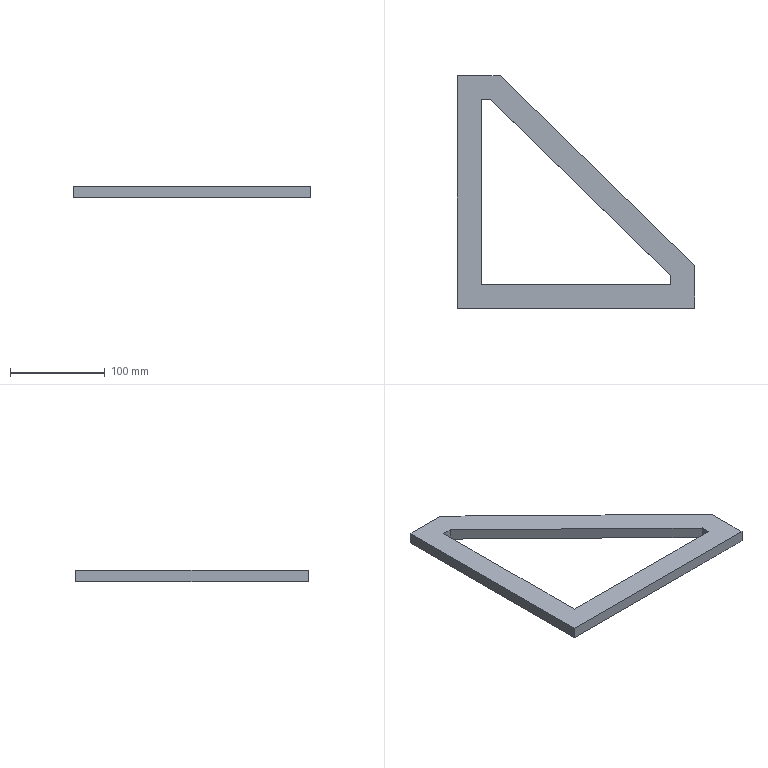Part | SolidWorks | features Extrusion 1 | 1 solid | 12 faces | box 250 x 245 x 12 mm | volume 232707 mm3 | plane 12
STEP:
#1=CARTESIAN_POINT('',(0.,0.,6.));
#2=VERTEX_POINT('',#1);
#3=CARTESIAN_POINT('',(0.,45.,6.));
#4=VERTEX_POINT('',#3);
#5=CARTESIAN_POINT('',(0.,45.,6.));
#6=DIRECTION('',(0.,1.,0.));
#7=VECTOR('',#6,1000.);
#8=LINE('',#5,#7);
#9=EDGE_CURVE('',#2,#4,#8,.T.);
#10=ORIENTED_EDGE('',*,*,#9,.T.);
#11=CARTESIAN_POINT('',(-205.,245.,6.));
#12=VERTEX_POINT('',#11);
#13=CARTESIAN_POINT('',(-205.,245.,6.));
#14=DIRECTION('',(-0.7158,0.6983,0.));
#15=VECTOR('',#14,1000.);
#16=LINE('',#13,#15);
#17=EDGE_CURVE('',#4,#12,#16,.T.);
#18=ORIENTED_EDGE('',*,*,#17,.T.);
#19=CARTESIAN_POINT('',(-250.,245.,6.));
#20=VERTEX_POINT('',#19);
#21=CARTESIAN_POINT('',(-250.,245.,6.));
#22=DIRECTION('',(-1.,0.,0.));
#23=VECTOR('',#22,1000.);
#24=LINE('',#21,#23);
#25=EDGE_CURVE('',#12,#20,#24,.T.);
#26=ORIENTED_EDGE('',*,*,#25,.T.);
#27=CARTESIAN_POINT('',(-250.,0.,6.));
#28=VERTEX_POINT('',#27);
#29=CARTESIAN_POINT('',(-250.,0.,6.));
#30=DIRECTION('',(0.,-1.,0.));
#31=VECTOR('',#30,1000.);
#32=LINE('',#29,#31);
#33=EDGE_CURVE('',#20,#28,#32,.T.);
#34=ORIENTED_EDGE('',*,*,#33,.T.);
#35=CARTESIAN_POINT('',(0.,0.,6.));
#36=DIRECTION('',(1.,0.,0.));
#37=VECTOR('',#36,1000.);
#38=LINE('',#35,#37);
#39=EDGE_CURVE('',#28,#2,#38,.T.);
#40=ORIENTED_EDGE('',*,*,#39,.T.);
#41=EDGE_LOOP('',(#10,#18,#26,#34,#40));
#42=FACE_OUTER_BOUND('',#41,.T.);
#43=CARTESIAN_POINT('',(-225.,220.,6.));
#44=VERTEX_POINT('',#43);
#45=CARTESIAN_POINT('',(-225.,25.,6.));
#46=VERTEX_POINT('',#45);
#47=CARTESIAN_POINT('',(-225.,25.,6.));
#48=DIRECTION('',(0.,-1.,0.));
#49=VECTOR('',#48,1000.);
#50=LINE('',#47,#49);
#51=EDGE_CURVE('',#44,#46,#50,.T.);
#52=ORIENTED_EDGE('',*,*,#51,.F.);
#53=CARTESIAN_POINT('',(-215.175,220.,6.));
#54=VERTEX_POINT('',#53);
#55=CARTESIAN_POINT('',(-225.,220.,6.));
#56=DIRECTION('',(-1.,0.,0.));
#57=VECTOR('',#56,1000.);
#58=LINE('',#55,#57);
#59=EDGE_CURVE('',#54,#44,#58,.T.);
#60=ORIENTED_EDGE('',*,*,#59,.F.);
#61=CARTESIAN_POINT('',(-25.,34.463,6.));
#62=VERTEX_POINT('',#61);
#63=CARTESIAN_POINT('',(-215.175,220.,6.));
#64=DIRECTION('',(-0.7158,0.6983,0.));
#65=VECTOR('',#64,1000.);
#66=LINE('',#63,#65);
#67=EDGE_CURVE('',#62,#54,#66,.T.);
#68=ORIENTED_EDGE('',*,*,#67,.F.);
#69=CARTESIAN_POINT('',(-25.,25.,6.));
#70=VERTEX_POINT('',#69);
#71=CARTESIAN_POINT('',(-25.,34.463,6.));
#72=DIRECTION('',(0.,1.,0.));
#73=VECTOR('',#72,1000.);
#74=LINE('',#71,#73);
#75=EDGE_CURVE('',#70,#62,#74,.T.);
#76=ORIENTED_EDGE('',*,*,#75,.F.);
#77=CARTESIAN_POINT('',(-25.,25.,6.));
#78=DIRECTION('',(1.,0.,0.));
#79=VECTOR('',#78,1000.);
#80=LINE('',#77,#79);
#81=EDGE_CURVE('',#46,#70,#80,.T.);
#82=ORIENTED_EDGE('',*,*,#81,.F.);
#83=EDGE_LOOP('',(#52,#60,#68,#76,#82));
#84=FACE_BOUND('',#83,.T.);
#85=CARTESIAN_POINT('',(0.,0.,6.));
#86=DIRECTION('',(0.,0.,-1.));
#87=DIRECTION('',(-1.,0.,0.));
#88=AXIS2_PLACEMENT_3D('',#85,#86,#87);
#89=PLANE('',#88);
#90=ADVANCED_FACE('',(#42,#84),#89,.F.);
#91=CARTESIAN_POINT('',(0.,0.,-6.));
#92=VERTEX_POINT('',#91);
#93=CARTESIAN_POINT('',(0.,45.,-6.));
#94=VERTEX_POINT('',#93);
#95=CARTESIAN_POINT('',(0.,45.,-6.));
#96=DIRECTION('',(0.,1.,0.));
#97=VECTOR('',#96,1000.);
#98=LINE('',#95,#97);
#99=EDGE_CURVE('',#92,#94,#98,.T.);
#100=ORIENTED_EDGE('',*,*,#99,.F.);
#101=CARTESIAN_POINT('',(-250.,0.,-6.));
#102=VERTEX_POINT('',#101);
#103=CARTESIAN_POINT('',(0.,0.,-6.));
#104=DIRECTION('',(1.,0.,0.));
#105=VECTOR('',#104,1000.);
#106=LINE('',#103,#105);
#107=EDGE_CURVE('',#102,#92,#106,.T.);
#108=ORIENTED_EDGE('',*,*,#107,.F.);
#109=CARTESIAN_POINT('',(-250.,245.,-6.));
#110=VERTEX_POINT('',#109);
#111=CARTESIAN_POINT('',(-250.,0.,-6.));
#112=DIRECTION('',(0.,-1.,0.));
#113=VECTOR('',#112,1000.);
#114=LINE('',#111,#113);
#115=EDGE_CURVE('',#110,#102,#114,.T.);
#116=ORIENTED_EDGE('',*,*,#115,.F.);
#117=CARTESIAN_POINT('',(-205.,245.,-6.));
#118=VERTEX_POINT('',#117);
#119=CARTESIAN_POINT('',(-250.,245.,-6.));
#120=DIRECTION('',(-1.,0.,0.));
#121=VECTOR('',#120,1000.);
#122=LINE('',#119,#121);
#123=EDGE_CURVE('',#118,#110,#122,.T.);
#124=ORIENTED_EDGE('',*,*,#123,.F.);
#125=CARTESIAN_POINT('',(-205.,245.,-6.));
#126=DIRECTION('',(-0.7158,0.6983,0.));
#127=VECTOR('',#126,1000.);
#128=LINE('',#125,#127);
#129=EDGE_CURVE('',#94,#118,#128,.T.);
#130=ORIENTED_EDGE('',*,*,#129,.F.);
#131=EDGE_LOOP('',(#100,#108,#116,#124,#130));
#132=FACE_OUTER_BOUND('',#131,.T.);
#133=CARTESIAN_POINT('',(-215.175,220.,-6.));
#134=VERTEX_POINT('',#133);
#135=CARTESIAN_POINT('',(-225.,220.,-6.));
#136=VERTEX_POINT('',#135);
#137=CARTESIAN_POINT('',(-225.,220.,-6.));
#138=DIRECTION('',(-1.,0.,0.));
#139=VECTOR('',#138,1000.);
#140=LINE('',#137,#139);
#141=EDGE_CURVE('',#134,#136,#140,.T.);
#142=ORIENTED_EDGE('',*,*,#141,.T.);
#143=CARTESIAN_POINT('',(-225.,25.,-6.));
#144=VERTEX_POINT('',#143);
#145=CARTESIAN_POINT('',(-225.,25.,-6.));
#146=DIRECTION('',(0.,-1.,0.));
#147=VECTOR('',#146,1000.);
#148=LINE('',#145,#147);
#149=EDGE_CURVE('',#136,#144,#148,.T.);
#150=ORIENTED_EDGE('',*,*,#149,.T.);
#151=CARTESIAN_POINT('',(-25.,25.,-6.));
#152=VERTEX_POINT('',#151);
#153=CARTESIAN_POINT('',(-25.,25.,-6.));
#154=DIRECTION('',(1.,0.,0.));
#155=VECTOR('',#154,1000.);
#156=LINE('',#153,#155);
#157=EDGE_CURVE('',#144,#152,#156,.T.);
#158=ORIENTED_EDGE('',*,*,#157,.T.);
#159=CARTESIAN_POINT('',(-25.,34.463,-6.));
#160=VERTEX_POINT('',#159);
#161=CARTESIAN_POINT('',(-25.,34.463,-6.));
#162=DIRECTION('',(0.,1.,0.));
#163=VECTOR('',#162,1000.);
#164=LINE('',#161,#163);
#165=EDGE_CURVE('',#152,#160,#164,.T.);
#166=ORIENTED_EDGE('',*,*,#165,.T.);
#167=CARTESIAN_POINT('',(-215.175,220.,-6.));
#168=DIRECTION('',(-0.7158,0.6983,0.));
#169=VECTOR('',#168,1000.);
#170=LINE('',#167,#169);
#171=EDGE_CURVE('',#160,#134,#170,.T.);
#172=ORIENTED_EDGE('',*,*,#171,.T.);
#173=EDGE_LOOP('',(#142,#150,#158,#166,#172));
#174=FACE_BOUND('',#173,.T.);
#175=CARTESIAN_POINT('',(0.,0.,-6.));
#176=DIRECTION('',(0.,0.,-1.));
#177=DIRECTION('',(-1.,0.,0.));
#178=AXIS2_PLACEMENT_3D('',#175,#176,#177);
#179=PLANE('',#178);
#180=ADVANCED_FACE('',(#132,#174),#179,.T.);
#181=ORIENTED_EDGE('',*,*,#99,.T.);
#182=CARTESIAN_POINT('',(0.,45.,6.));
#183=DIRECTION('',(0.,0.,-1.));
#184=VECTOR('',#183,1000.);
#185=LINE('',#182,#184);
#186=EDGE_CURVE('',#4,#94,#185,.T.);
#187=ORIENTED_EDGE('',*,*,#186,.F.);
#188=ORIENTED_EDGE('',*,*,#9,.F.);
#189=CARTESIAN_POINT('',(0.,0.,6.));
#190=DIRECTION('',(0.,0.,-1.));
#191=VECTOR('',#190,1000.);
#192=LINE('',#189,#191);
#193=EDGE_CURVE('',#2,#92,#192,.T.);
#194=ORIENTED_EDGE('',*,*,#193,.T.);
#195=EDGE_LOOP('',(#181,#187,#188,#194));
#196=FACE_OUTER_BOUND('',#195,.T.);
#197=CARTESIAN_POINT('',(0.,45.,6.));
#198=DIRECTION('',(-1.,0.,0.));
#199=DIRECTION('',(0.,-1.,0.));
#200=AXIS2_PLACEMENT_3D('',#197,#198,#199);
#201=PLANE('',#200);
#202=ADVANCED_FACE('',(#196),#201,.F.);
#203=ORIENTED_EDGE('',*,*,#129,.T.);
#204=CARTESIAN_POINT('',(-205.,245.,6.));
#205=DIRECTION('',(0.,0.,-1.));
#206=VECTOR('',#205,1000.);
#207=LINE('',#204,#206);
#208=EDGE_CURVE('',#12,#118,#207,.T.);
#209=ORIENTED_EDGE('',*,*,#208,.F.);
#210=ORIENTED_EDGE('',*,*,#17,.F.);
#211=ORIENTED_EDGE('',*,*,#186,.T.);
#212=EDGE_LOOP('',(#203,#209,#210,#211));
#213=FACE_OUTER_BOUND('',#212,.T.);
#214=CARTESIAN_POINT('',(-205.,245.,6.));
#215=DIRECTION('',(-0.6983,-0.7158,0.));
#216=DIRECTION('',(0.7158,-0.6983,0.));
#217=AXIS2_PLACEMENT_3D('',#214,#215,#216);
#218=PLANE('',#217);
#219=ADVANCED_FACE('',(#213),#218,.F.);
#220=ORIENTED_EDGE('',*,*,#123,.T.);
#221=CARTESIAN_POINT('',(-250.,245.,6.));
#222=DIRECTION('',(0.,0.,-1.));
#223=VECTOR('',#222,1000.);
#224=LINE('',#221,#223);
#225=EDGE_CURVE('',#20,#110,#224,.T.);
#226=ORIENTED_EDGE('',*,*,#225,.F.);
#227=ORIENTED_EDGE('',*,*,#25,.F.);
#228=ORIENTED_EDGE('',*,*,#208,.T.);
#229=EDGE_LOOP('',(#220,#226,#227,#228));
#230=FACE_OUTER_BOUND('',#229,.T.);
#231=CARTESIAN_POINT('',(-250.,245.,6.));
#232=DIRECTION('',(0.,-1.,0.));
#233=DIRECTION('',(0.,0.,-1.));
#234=AXIS2_PLACEMENT_3D('',#231,#232,#233);
#235=PLANE('',#234);
#236=ADVANCED_FACE('',(#230),#235,.F.);
#237=ORIENTED_EDGE('',*,*,#115,.T.);
#238=CARTESIAN_POINT('',(-250.,0.,6.));
#239=DIRECTION('',(0.,0.,-1.));
#240=VECTOR('',#239,1000.);
#241=LINE('',#238,#240);
#242=EDGE_CURVE('',#28,#102,#241,.T.);
#243=ORIENTED_EDGE('',*,*,#242,.F.);
#244=ORIENTED_EDGE('',*,*,#33,.F.);
#245=ORIENTED_EDGE('',*,*,#225,.T.);
#246=EDGE_LOOP('',(#237,#243,#244,#245));
#247=FACE_OUTER_BOUND('',#246,.T.);
#248=CARTESIAN_POINT('',(-250.,0.,6.));
#249=DIRECTION('',(1.,0.,0.));
#250=DIRECTION('',(0.,0.,-1.));
#251=AXIS2_PLACEMENT_3D('',#248,#249,#250);
#252=PLANE('',#251);
#253=ADVANCED_FACE('',(#247),#252,.F.);
#254=ORIENTED_EDGE('',*,*,#107,.T.);
#255=ORIENTED_EDGE('',*,*,#193,.F.);
#256=ORIENTED_EDGE('',*,*,#39,.F.);
#257=ORIENTED_EDGE('',*,*,#242,.T.);
#258=EDGE_LOOP('',(#254,#255,#256,#257));
#259=FACE_OUTER_BOUND('',#258,.T.);
#260=CARTESIAN_POINT('',(0.,0.,6.));
#261=DIRECTION('',(0.,1.,0.));
#262=DIRECTION('',(-1.,0.,0.));
#263=AXIS2_PLACEMENT_3D('',#260,#261,#262);
#264=PLANE('',#263);
#265=ADVANCED_FACE('',(#259),#264,.F.);
#266=ORIENTED_EDGE('',*,*,#149,.F.);
#267=CARTESIAN_POINT('',(-225.,220.,6.));
#268=DIRECTION('',(0.,0.,-1.));
#269=VECTOR('',#268,1000.);
#270=LINE('',#267,#269);
#271=EDGE_CURVE('',#44,#136,#270,.T.);
#272=ORIENTED_EDGE('',*,*,#271,.F.);
#273=ORIENTED_EDGE('',*,*,#51,.T.);
#274=CARTESIAN_POINT('',(-225.,25.,6.));
#275=DIRECTION('',(0.,0.,-1.));
#276=VECTOR('',#275,1000.);
#277=LINE('',#274,#276);
#278=EDGE_CURVE('',#46,#144,#277,.T.);
#279=ORIENTED_EDGE('',*,*,#278,.T.);
#280=EDGE_LOOP('',(#266,#272,#273,#279));
#281=FACE_OUTER_BOUND('',#280,.T.);
#282=CARTESIAN_POINT('',(-225.,25.,6.));
#283=DIRECTION('',(1.,0.,0.));
#284=DIRECTION('',(0.,0.,-1.));
#285=AXIS2_PLACEMENT_3D('',#282,#283,#284);
#286=PLANE('',#285);
#287=ADVANCED_FACE('',(#281),#286,.T.);
#288=ORIENTED_EDGE('',*,*,#157,.F.);
#289=ORIENTED_EDGE('',*,*,#278,.F.);
#290=ORIENTED_EDGE('',*,*,#81,.T.);
#291=CARTESIAN_POINT('',(-25.,25.,6.));
#292=DIRECTION('',(0.,0.,-1.));
#293=VECTOR('',#292,1000.);
#294=LINE('',#291,#293);
#295=EDGE_CURVE('',#70,#152,#294,.T.);
#296=ORIENTED_EDGE('',*,*,#295,.T.);
#297=EDGE_LOOP('',(#288,#289,#290,#296));
#298=FACE_OUTER_BOUND('',#297,.T.);
#299=CARTESIAN_POINT('',(-25.,25.,6.));
#300=DIRECTION('',(0.,1.,0.));
#301=DIRECTION('',(-1.,0.,0.));
#302=AXIS2_PLACEMENT_3D('',#299,#300,#301);
#303=PLANE('',#302);
#304=ADVANCED_FACE('',(#298),#303,.T.);
#305=ORIENTED_EDGE('',*,*,#165,.F.);
#306=ORIENTED_EDGE('',*,*,#295,.F.);
#307=ORIENTED_EDGE('',*,*,#75,.T.);
#308=CARTESIAN_POINT('',(-25.,34.463,6.));
#309=DIRECTION('',(0.,0.,-1.));
#310=VECTOR('',#309,1000.);
#311=LINE('',#308,#310);
#312=EDGE_CURVE('',#62,#160,#311,.T.);
#313=ORIENTED_EDGE('',*,*,#312,.T.);
#314=EDGE_LOOP('',(#305,#306,#307,#313));
#315=FACE_OUTER_BOUND('',#314,.T.);
#316=CARTESIAN_POINT('',(-25.,34.463,6.));
#317=DIRECTION('',(-1.,0.,0.));
#318=DIRECTION('',(0.,0.,1.));
#319=AXIS2_PLACEMENT_3D('',#316,#317,#318);
#320=PLANE('',#319);
#321=ADVANCED_FACE('',(#315),#320,.T.);
#322=ORIENTED_EDGE('',*,*,#171,.F.);
#323=ORIENTED_EDGE('',*,*,#312,.F.);
#324=ORIENTED_EDGE('',*,*,#67,.T.);
#325=CARTESIAN_POINT('',(-215.175,220.,6.));
#326=DIRECTION('',(0.,0.,-1.));
#327=VECTOR('',#326,1000.);
#328=LINE('',#325,#327);
#329=EDGE_CURVE('',#54,#134,#328,.T.);
#330=ORIENTED_EDGE('',*,*,#329,.T.);
#331=EDGE_LOOP('',(#322,#323,#324,#330));
#332=FACE_OUTER_BOUND('',#331,.T.);
#333=CARTESIAN_POINT('',(-215.175,220.,6.));
#334=DIRECTION('',(-0.6983,-0.7158,0.));
#335=DIRECTION('',(0.7158,-0.6983,0.));
#336=AXIS2_PLACEMENT_3D('',#333,#334,#335);
#337=PLANE('',#336);
#338=ADVANCED_FACE('',(#332),#337,.T.);
#339=ORIENTED_EDGE('',*,*,#141,.F.);
#340=ORIENTED_EDGE('',*,*,#329,.F.);
#341=ORIENTED_EDGE('',*,*,#59,.T.);
#342=ORIENTED_EDGE('',*,*,#271,.T.);
#343=EDGE_LOOP('',(#339,#340,#341,#342));
#344=FACE_OUTER_BOUND('',#343,.T.);
#345=CARTESIAN_POINT('',(-225.,220.,6.));
#346=DIRECTION('',(0.,-1.,0.));
#347=DIRECTION('',(0.,0.,-1.));
#348=AXIS2_PLACEMENT_3D('',#345,#346,#347);
#349=PLANE('',#348);
#350=ADVANCED_FACE('',(#344),#349,.T.);
#351=CLOSED_SHELL('',(#90,#180,#202,#219,#236,#253,#265,#287,#304,#321,#338,#350));
#352=MANIFOLD_SOLID_BREP('',#351);
#353=CARTESIAN_POINT('',(0.,0.,0.));
#354=DIRECTION('',(0.,0.,1.));
#355=DIRECTION('',(1.,0.,0.));
#356=AXIS2_PLACEMENT_3D('',#353,#354,#355);
#357=(LENGTH_UNIT()NAMED_UNIT(*)SI_UNIT(.MILLI.,.METRE.));
#358=UNCERTAINTY_MEASURE_WITH_UNIT(LENGTH_MEASURE(0.00001),#357,'','');
#359=(NAMED_UNIT(*)PLANE_ANGLE_UNIT()SI_UNIT($,.RADIAN.));
#360=(NAMED_UNIT(*)SI_UNIT($,.STERADIAN.)SOLID_ANGLE_UNIT());
#361=(GEOMETRIC_REPRESENTATION_CONTEXT(3)GLOBAL_UNCERTAINTY_ASSIGNED_CONTEXT((#358))GLOBAL_UNIT_ASSIGNED_CONTEXT((#357,#359,#360))REPRESENTATION_CONTEXT('',''));
#362=ADVANCED_BREP_SHAPE_REPRESENTATION('',(#352,#356),#361);